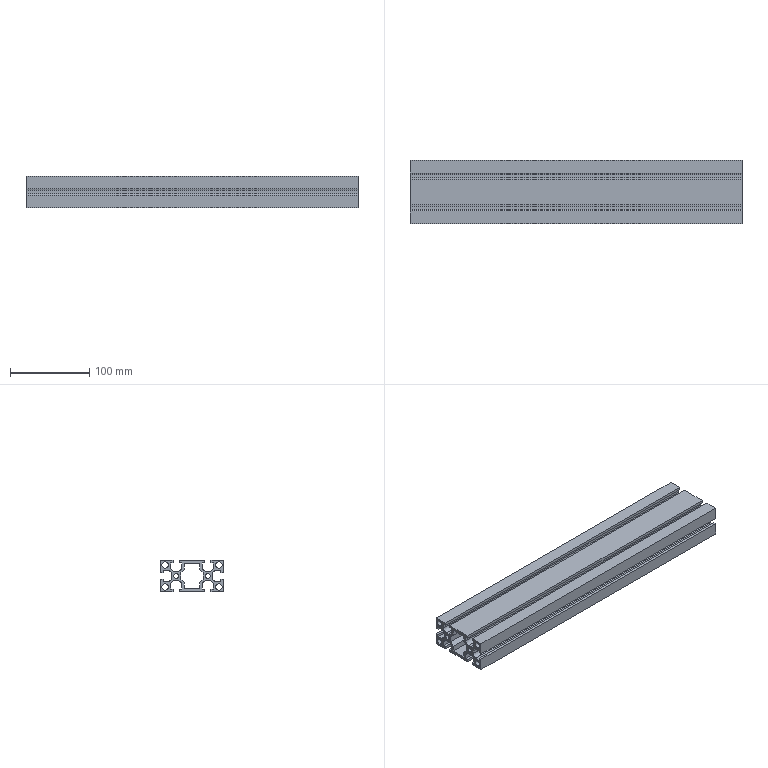Part | SolidWorks | features BaseBody 1 | 1 solid | 90 faces | box 420 x 80 x 40 mm | volume 517624 mm3 | plane 66 | cylinder 24 | commonest cylinder face diameters 10 x12 8 x8 6.2 x4